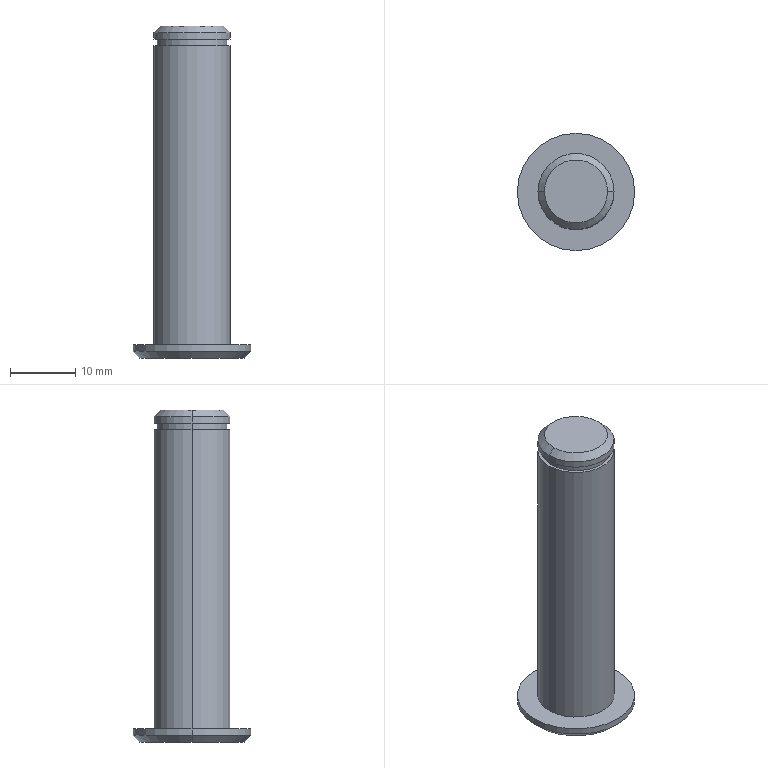Part | SolidWorks | features ICE 3, Chamfer 1, Extrusion 1 | 1 solid | 17 faces | box 18 x 18 x 51 mm | volume 5715 mm3 | cylinder 8 | plane 5 | cone 4 | commonest cylinder face diameters 11.7 x4 10.7 x2 18 x2
STEP:
#1=CARTESIAN_POINT('',(4.85,0.,51.));
#2=VERTEX_POINT('',#1);
#3=CARTESIAN_POINT('',(-4.85,0.,51.));
#4=VERTEX_POINT('',#3);
#5=CARTESIAN_POINT('',(0.,0.,51.));
#6=DIRECTION('',(0.,0.,1.));
#7=DIRECTION('',(1.,0.,0.));
#8=AXIS2_PLACEMENT_3D('',#5,#6,#7);
#9=CIRCLE('',#8,4.85);
#10=EDGE_CURVE('',#2,#4,#9,.T.);
#11=ORIENTED_EDGE('',*,*,#10,.F.);
#12=CARTESIAN_POINT('',(5.85,0.,50.));
#13=VERTEX_POINT('',#12);
#14=CARTESIAN_POINT('',(4.85,0.,51.));
#15=DIRECTION('',(0.7071,0.,-0.7071));
#16=VECTOR('',#15,1000.);
#17=LINE('',#14,#16);
#18=EDGE_CURVE('',#2,#13,#17,.T.);
#19=ORIENTED_EDGE('',*,*,#18,.T.);
#20=CARTESIAN_POINT('',(-5.85,0.,50.));
#21=VERTEX_POINT('',#20);
#22=CARTESIAN_POINT('',(0.,0.,50.));
#23=DIRECTION('',(0.,0.,-1.));
#24=DIRECTION('',(1.,0.,0.));
#25=AXIS2_PLACEMENT_3D('',#22,#23,#24);
#26=CIRCLE('',#25,5.85);
#27=EDGE_CURVE('',#21,#13,#26,.T.);
#28=ORIENTED_EDGE('',*,*,#27,.F.);
#29=CARTESIAN_POINT('',(-4.85,0.,51.));
#30=DIRECTION('',(-0.7071,0.,-0.7071));
#31=VECTOR('',#30,1000.);
#32=LINE('',#29,#31);
#33=EDGE_CURVE('',#4,#21,#32,.T.);
#34=ORIENTED_EDGE('',*,*,#33,.F.);
#35=EDGE_LOOP('',(#11,#19,#28,#34));
#36=FACE_OUTER_BOUND('',#35,.T.);
#37=CARTESIAN_POINT('',(0.,0.,51.));
#38=DIRECTION('',(0.,0.,-1.));
#39=DIRECTION('',(-1.,0.,0.));
#40=AXIS2_PLACEMENT_3D('',#37,#38,#39);
#41=CONICAL_SURFACE('',#40,4.85,0.7854);
#42=ADVANCED_FACE('',(#36),#41,.T.);
#43=CARTESIAN_POINT('',(-8.,0.,0.));
#44=VERTEX_POINT('',#43);
#45=CARTESIAN_POINT('',(8.,0.,0.));
#46=VERTEX_POINT('',#45);
#47=CARTESIAN_POINT('',(0.,0.,0.));
#48=DIRECTION('',(0.,0.,-1.));
#49=DIRECTION('',(1.,0.,0.));
#50=AXIS2_PLACEMENT_3D('',#47,#48,#49);
#51=CIRCLE('',#50,8.);
#52=EDGE_CURVE('',#44,#46,#51,.T.);
#53=ORIENTED_EDGE('',*,*,#52,.F.);
#54=CARTESIAN_POINT('',(-9.,0.,1.));
#55=VERTEX_POINT('',#54);
#56=CARTESIAN_POINT('',(-9.,0.,1.));
#57=DIRECTION('',(-0.7071,0.,0.7071));
#58=VECTOR('',#57,1000.);
#59=LINE('',#56,#58);
#60=EDGE_CURVE('',#44,#55,#59,.T.);
#61=ORIENTED_EDGE('',*,*,#60,.T.);
#62=CARTESIAN_POINT('',(9.,0.,1.));
#63=VERTEX_POINT('',#62);
#64=CARTESIAN_POINT('',(0.,0.,1.));
#65=DIRECTION('',(0.,0.,1.));
#66=DIRECTION('',(1.,0.,0.));
#67=AXIS2_PLACEMENT_3D('',#64,#65,#66);
#68=CIRCLE('',#67,9.);
#69=EDGE_CURVE('',#63,#55,#68,.T.);
#70=ORIENTED_EDGE('',*,*,#69,.F.);
#71=CARTESIAN_POINT('',(9.,0.,1.));
#72=DIRECTION('',(0.7071,0.,0.7071));
#73=VECTOR('',#72,1000.);
#74=LINE('',#71,#73);
#75=EDGE_CURVE('',#46,#63,#74,.T.);
#76=ORIENTED_EDGE('',*,*,#75,.F.);
#77=EDGE_LOOP('',(#53,#61,#70,#76));
#78=FACE_OUTER_BOUND('',#77,.T.);
#79=CARTESIAN_POINT('',(0.,0.,1.));
#80=DIRECTION('',(0.,0.,1.));
#81=DIRECTION('',(1.,0.,0.));
#82=AXIS2_PLACEMENT_3D('',#79,#80,#81);
#83=CONICAL_SURFACE('',#82,9.,0.7854);
#84=ADVANCED_FACE('',(#78),#83,.T.);
#85=ORIENTED_EDGE('',*,*,#27,.T.);
#86=CARTESIAN_POINT('',(5.85,0.,49.));
#87=VERTEX_POINT('',#86);
#88=CARTESIAN_POINT('',(5.85,0.,51.));
#89=DIRECTION('',(0.,0.,-1.));
#90=VECTOR('',#89,1000.);
#91=LINE('',#88,#90);
#92=EDGE_CURVE('',#13,#87,#91,.T.);
#93=ORIENTED_EDGE('',*,*,#92,.T.);
#94=CARTESIAN_POINT('',(-5.85,0.,49.));
#95=VERTEX_POINT('',#94);
#96=CARTESIAN_POINT('',(0.,0.,49.));
#97=DIRECTION('',(0.,0.,1.));
#98=DIRECTION('',(1.,0.,0.));
#99=AXIS2_PLACEMENT_3D('',#96,#97,#98);
#100=CIRCLE('',#99,5.85);
#101=EDGE_CURVE('',#87,#95,#100,.T.);
#102=ORIENTED_EDGE('',*,*,#101,.T.);
#103=CARTESIAN_POINT('',(-5.85,0.,51.));
#104=DIRECTION('',(0.,0.,-1.));
#105=VECTOR('',#104,1000.);
#106=LINE('',#103,#105);
#107=EDGE_CURVE('',#21,#95,#106,.T.);
#108=ORIENTED_EDGE('',*,*,#107,.F.);
#109=EDGE_LOOP('',(#85,#93,#102,#108));
#110=FACE_OUTER_BOUND('',#109,.T.);
#111=CARTESIAN_POINT('',(0.,0.,51.));
#112=DIRECTION('',(0.,0.,-1.));
#113=DIRECTION('',(-1.,0.,0.));
#114=AXIS2_PLACEMENT_3D('',#111,#112,#113);
#115=CYLINDRICAL_SURFACE('',#114,5.85);
#116=ADVANCED_FACE('',(#110),#115,.T.);
#117=CARTESIAN_POINT('',(5.35,0.,49.));
#118=VERTEX_POINT('',#117);
#119=CARTESIAN_POINT('',(-5.35,0.,49.));
#120=VERTEX_POINT('',#119);
#121=CARTESIAN_POINT('',(0.,0.,49.));
#122=DIRECTION('',(0.,0.,1.));
#123=DIRECTION('',(1.,0.,0.));
#124=AXIS2_PLACEMENT_3D('',#121,#122,#123);
#125=CIRCLE('',#124,5.35);
#126=EDGE_CURVE('',#118,#120,#125,.T.);
#127=ORIENTED_EDGE('',*,*,#126,.F.);
#128=CARTESIAN_POINT('',(5.35,0.,48.));
#129=VERTEX_POINT('',#128);
#130=CARTESIAN_POINT('',(5.35,0.,49.));
#131=DIRECTION('',(0.,0.,-1.));
#132=VECTOR('',#131,1000.);
#133=LINE('',#130,#132);
#134=EDGE_CURVE('',#118,#129,#133,.T.);
#135=ORIENTED_EDGE('',*,*,#134,.T.);
#136=CARTESIAN_POINT('',(-5.35,0.,48.));
#137=VERTEX_POINT('',#136);
#138=CARTESIAN_POINT('',(0.,0.,48.));
#139=DIRECTION('',(0.,0.,1.));
#140=DIRECTION('',(1.,0.,0.));
#141=AXIS2_PLACEMENT_3D('',#138,#139,#140);
#142=CIRCLE('',#141,5.35);
#143=EDGE_CURVE('',#129,#137,#142,.T.);
#144=ORIENTED_EDGE('',*,*,#143,.T.);
#145=CARTESIAN_POINT('',(-5.35,0.,49.));
#146=DIRECTION('',(0.,0.,-1.));
#147=VECTOR('',#146,1000.);
#148=LINE('',#145,#147);
#149=EDGE_CURVE('',#120,#137,#148,.T.);
#150=ORIENTED_EDGE('',*,*,#149,.F.);
#151=EDGE_LOOP('',(#127,#135,#144,#150));
#152=FACE_OUTER_BOUND('',#151,.T.);
#153=CARTESIAN_POINT('',(0.,0.,49.));
#154=DIRECTION('',(0.,0.,-1.));
#155=DIRECTION('',(-1.,0.,0.));
#156=AXIS2_PLACEMENT_3D('',#153,#154,#155);
#157=CYLINDRICAL_SURFACE('',#156,5.35);
#158=ADVANCED_FACE('',(#152),#157,.T.);
#159=CARTESIAN_POINT('',(5.85,0.,48.));
#160=VERTEX_POINT('',#159);
#161=CARTESIAN_POINT('',(-5.85,0.,48.));
#162=VERTEX_POINT('',#161);
#163=CARTESIAN_POINT('',(0.,0.,48.));
#164=DIRECTION('',(0.,0.,1.));
#165=DIRECTION('',(1.,0.,0.));
#166=AXIS2_PLACEMENT_3D('',#163,#164,#165);
#167=CIRCLE('',#166,5.85);
#168=EDGE_CURVE('',#160,#162,#167,.T.);
#169=ORIENTED_EDGE('',*,*,#168,.F.);
#170=CARTESIAN_POINT('',(5.85,0.,2.));
#171=VERTEX_POINT('',#170);
#172=CARTESIAN_POINT('',(5.85,0.,48.));
#173=DIRECTION('',(0.,0.,-1.));
#174=VECTOR('',#173,1000.);
#175=LINE('',#172,#174);
#176=EDGE_CURVE('',#160,#171,#175,.T.);
#177=ORIENTED_EDGE('',*,*,#176,.T.);
#178=CARTESIAN_POINT('',(-5.85,0.,2.));
#179=VERTEX_POINT('',#178);
#180=CARTESIAN_POINT('',(0.,0.,2.));
#181=DIRECTION('',(0.,0.,1.));
#182=DIRECTION('',(1.,0.,0.));
#183=AXIS2_PLACEMENT_3D('',#180,#181,#182);
#184=CIRCLE('',#183,5.85);
#185=EDGE_CURVE('',#171,#179,#184,.T.);
#186=ORIENTED_EDGE('',*,*,#185,.T.);
#187=CARTESIAN_POINT('',(-5.85,0.,48.));
#188=DIRECTION('',(0.,0.,-1.));
#189=VECTOR('',#188,1000.);
#190=LINE('',#187,#189);
#191=EDGE_CURVE('',#162,#179,#190,.T.);
#192=ORIENTED_EDGE('',*,*,#191,.F.);
#193=EDGE_LOOP('',(#169,#177,#186,#192));
#194=FACE_OUTER_BOUND('',#193,.T.);
#195=CARTESIAN_POINT('',(0.,0.,48.));
#196=DIRECTION('',(0.,0.,-1.));
#197=DIRECTION('',(-1.,0.,0.));
#198=AXIS2_PLACEMENT_3D('',#195,#196,#197);
#199=CYLINDRICAL_SURFACE('',#198,5.85);
#200=ADVANCED_FACE('',(#194),#199,.T.);
#201=CARTESIAN_POINT('',(9.,0.,2.));
#202=VERTEX_POINT('',#201);
#203=CARTESIAN_POINT('',(-9.,0.,2.));
#204=VERTEX_POINT('',#203);
#205=CARTESIAN_POINT('',(0.,0.,2.));
#206=DIRECTION('',(0.,0.,1.));
#207=DIRECTION('',(1.,0.,0.));
#208=AXIS2_PLACEMENT_3D('',#205,#206,#207);
#209=CIRCLE('',#208,9.);
#210=EDGE_CURVE('',#202,#204,#209,.T.);
#211=ORIENTED_EDGE('',*,*,#210,.F.);
#212=CARTESIAN_POINT('',(9.,0.,2.));
#213=DIRECTION('',(0.,0.,-1.));
#214=VECTOR('',#213,1000.);
#215=LINE('',#212,#214);
#216=EDGE_CURVE('',#202,#63,#215,.T.);
#217=ORIENTED_EDGE('',*,*,#216,.T.);
#218=ORIENTED_EDGE('',*,*,#69,.T.);
#219=CARTESIAN_POINT('',(-9.,0.,2.));
#220=DIRECTION('',(0.,0.,-1.));
#221=VECTOR('',#220,1000.);
#222=LINE('',#219,#221);
#223=EDGE_CURVE('',#204,#55,#222,.T.);
#224=ORIENTED_EDGE('',*,*,#223,.F.);
#225=EDGE_LOOP('',(#211,#217,#218,#224));
#226=FACE_OUTER_BOUND('',#225,.T.);
#227=CARTESIAN_POINT('',(0.,0.,2.));
#228=DIRECTION('',(0.,0.,-1.));
#229=DIRECTION('',(-1.,0.,0.));
#230=AXIS2_PLACEMENT_3D('',#227,#228,#229);
#231=CYLINDRICAL_SURFACE('',#230,9.);
#232=ADVANCED_FACE('',(#226),#231,.T.);
#233=ORIENTED_EDGE('',*,*,#216,.F.);
#234=CARTESIAN_POINT('',(0.,0.,2.));
#235=DIRECTION('',(0.,0.,1.));
#236=DIRECTION('',(1.,0.,0.));
#237=AXIS2_PLACEMENT_3D('',#234,#235,#236);
#238=CIRCLE('',#237,9.);
#239=EDGE_CURVE('',#204,#202,#238,.T.);
#240=ORIENTED_EDGE('',*,*,#239,.F.);
#241=ORIENTED_EDGE('',*,*,#223,.T.);
#242=CARTESIAN_POINT('',(0.,0.,1.));
#243=DIRECTION('',(0.,0.,1.));
#244=DIRECTION('',(1.,0.,0.));
#245=AXIS2_PLACEMENT_3D('',#242,#243,#244);
#246=CIRCLE('',#245,9.);
#247=EDGE_CURVE('',#55,#63,#246,.T.);
#248=ORIENTED_EDGE('',*,*,#247,.T.);
#249=EDGE_LOOP('',(#233,#240,#241,#248));
#250=FACE_OUTER_BOUND('',#249,.T.);
#251=CARTESIAN_POINT('',(0.,0.,2.));
#252=DIRECTION('',(0.,0.,-1.));
#253=DIRECTION('',(-1.,0.,0.));
#254=AXIS2_PLACEMENT_3D('',#251,#252,#253);
#255=CYLINDRICAL_SURFACE('',#254,9.);
#256=ADVANCED_FACE('',(#250),#255,.T.);
#257=CARTESIAN_POINT('',(0.,0.,2.));
#258=DIRECTION('',(0.,0.,1.));
#259=DIRECTION('',(1.,0.,0.));
#260=AXIS2_PLACEMENT_3D('',#257,#258,#259);
#261=CIRCLE('',#260,5.85);
#262=EDGE_CURVE('',#179,#171,#261,.T.);
#263=ORIENTED_EDGE('',*,*,#262,.F.);
#264=ORIENTED_EDGE('',*,*,#185,.F.);
#265=EDGE_LOOP('',(#263,#264));
#266=FACE_BOUND('',#265,.T.);
#267=ORIENTED_EDGE('',*,*,#239,.T.);
#268=ORIENTED_EDGE('',*,*,#210,.T.);
#269=EDGE_LOOP('',(#267,#268));
#270=FACE_OUTER_BOUND('',#269,.T.);
#271=CARTESIAN_POINT('',(0.,0.,2.));
#272=DIRECTION('',(0.,0.,1.));
#273=DIRECTION('',(1.,0.,0.));
#274=AXIS2_PLACEMENT_3D('',#271,#272,#273);
#275=PLANE('',#274);
#276=ADVANCED_FACE('',(#266,#270),#275,.T.);
#277=CARTESIAN_POINT('',(0.,0.,0.));
#278=DIRECTION('',(0.,0.,-1.));
#279=DIRECTION('',(1.,0.,0.));
#280=AXIS2_PLACEMENT_3D('',#277,#278,#279);
#281=CIRCLE('',#280,8.);
#282=EDGE_CURVE('',#46,#44,#281,.T.);
#283=ORIENTED_EDGE('',*,*,#282,.T.);
#284=ORIENTED_EDGE('',*,*,#52,.T.);
#285=EDGE_LOOP('',(#283,#284));
#286=FACE_OUTER_BOUND('',#285,.T.);
#287=CARTESIAN_POINT('',(0.,0.,0.));
#288=DIRECTION('',(0.,0.,1.));
#289=DIRECTION('',(1.,0.,0.));
#290=AXIS2_PLACEMENT_3D('',#287,#288,#289);
#291=PLANE('',#290);
#292=ADVANCED_FACE('',(#286),#291,.F.);
#293=ORIENTED_EDGE('',*,*,#176,.F.);
#294=CARTESIAN_POINT('',(0.,0.,48.));
#295=DIRECTION('',(0.,0.,1.));
#296=DIRECTION('',(1.,0.,0.));
#297=AXIS2_PLACEMENT_3D('',#294,#295,#296);
#298=CIRCLE('',#297,5.85);
#299=EDGE_CURVE('',#162,#160,#298,.T.);
#300=ORIENTED_EDGE('',*,*,#299,.F.);
#301=ORIENTED_EDGE('',*,*,#191,.T.);
#302=ORIENTED_EDGE('',*,*,#262,.T.);
#303=EDGE_LOOP('',(#293,#300,#301,#302));
#304=FACE_OUTER_BOUND('',#303,.T.);
#305=CARTESIAN_POINT('',(0.,0.,48.));
#306=DIRECTION('',(0.,0.,-1.));
#307=DIRECTION('',(-1.,0.,0.));
#308=AXIS2_PLACEMENT_3D('',#305,#306,#307);
#309=CYLINDRICAL_SURFACE('',#308,5.85);
#310=ADVANCED_FACE('',(#304),#309,.T.);
#311=CARTESIAN_POINT('',(0.,0.,48.));
#312=DIRECTION('',(0.,0.,1.));
#313=DIRECTION('',(1.,0.,0.));
#314=AXIS2_PLACEMENT_3D('',#311,#312,#313);
#315=CIRCLE('',#314,5.35);
#316=EDGE_CURVE('',#137,#129,#315,.T.);
#317=ORIENTED_EDGE('',*,*,#316,.F.);
#318=ORIENTED_EDGE('',*,*,#143,.F.);
#319=EDGE_LOOP('',(#317,#318));
#320=FACE_BOUND('',#319,.T.);
#321=ORIENTED_EDGE('',*,*,#299,.T.);
#322=ORIENTED_EDGE('',*,*,#168,.T.);
#323=EDGE_LOOP('',(#321,#322));
#324=FACE_OUTER_BOUND('',#323,.T.);
#325=CARTESIAN_POINT('',(0.,0.,48.));
#326=DIRECTION('',(0.,0.,1.));
#327=DIRECTION('',(1.,0.,0.));
#328=AXIS2_PLACEMENT_3D('',#325,#326,#327);
#329=PLANE('',#328);
#330=ADVANCED_FACE('',(#320,#324),#329,.T.);
#331=ORIENTED_EDGE('',*,*,#134,.F.);
#332=CARTESIAN_POINT('',(0.,0.,49.));
#333=DIRECTION('',(0.,0.,1.));
#334=DIRECTION('',(1.,0.,0.));
#335=AXIS2_PLACEMENT_3D('',#332,#333,#334);
#336=CIRCLE('',#335,5.35);
#337=EDGE_CURVE('',#120,#118,#336,.T.);
#338=ORIENTED_EDGE('',*,*,#337,.F.);
#339=ORIENTED_EDGE('',*,*,#149,.T.);
#340=ORIENTED_EDGE('',*,*,#316,.T.);
#341=EDGE_LOOP('',(#331,#338,#339,#340));
#342=FACE_OUTER_BOUND('',#341,.T.);
#343=CARTESIAN_POINT('',(0.,0.,49.));
#344=DIRECTION('',(0.,0.,-1.));
#345=DIRECTION('',(-1.,0.,0.));
#346=AXIS2_PLACEMENT_3D('',#343,#344,#345);
#347=CYLINDRICAL_SURFACE('',#346,5.35);
#348=ADVANCED_FACE('',(#342),#347,.T.);
#349=ORIENTED_EDGE('',*,*,#92,.F.);
#350=CARTESIAN_POINT('',(0.,0.,50.));
#351=DIRECTION('',(0.,0.,-1.));
#352=DIRECTION('',(1.,0.,0.));
#353=AXIS2_PLACEMENT_3D('',#350,#351,#352);
#354=CIRCLE('',#353,5.85);
#355=EDGE_CURVE('',#13,#21,#354,.T.);
#356=ORIENTED_EDGE('',*,*,#355,.T.);
#357=ORIENTED_EDGE('',*,*,#107,.T.);
#358=CARTESIAN_POINT('',(0.,0.,49.));
#359=DIRECTION('',(0.,0.,1.));
#360=DIRECTION('',(1.,0.,0.));
#361=AXIS2_PLACEMENT_3D('',#358,#359,#360);
#362=CIRCLE('',#361,5.85);
#363=EDGE_CURVE('',#95,#87,#362,.T.);
#364=ORIENTED_EDGE('',*,*,#363,.T.);
#365=EDGE_LOOP('',(#349,#356,#357,#364));
#366=FACE_OUTER_BOUND('',#365,.T.);
#367=CARTESIAN_POINT('',(0.,0.,51.));
#368=DIRECTION('',(0.,0.,-1.));
#369=DIRECTION('',(-1.,0.,0.));
#370=AXIS2_PLACEMENT_3D('',#367,#368,#369);
#371=CYLINDRICAL_SURFACE('',#370,5.85);
#372=ADVANCED_FACE('',(#366),#371,.T.);
#373=CARTESIAN_POINT('',(0.,0.,51.));
#374=DIRECTION('',(0.,0.,1.));
#375=DIRECTION('',(1.,0.,0.));
#376=AXIS2_PLACEMENT_3D('',#373,#374,#375);
#377=CIRCLE('',#376,4.85);
#378=EDGE_CURVE('',#4,#2,#377,.T.);
#379=ORIENTED_EDGE('',*,*,#378,.T.);
#380=ORIENTED_EDGE('',*,*,#10,.T.);
#381=EDGE_LOOP('',(#379,#380));
#382=FACE_OUTER_BOUND('',#381,.T.);
#383=CARTESIAN_POINT('',(0.,0.,51.));
#384=DIRECTION('',(0.,0.,1.));
#385=DIRECTION('',(1.,0.,0.));
#386=AXIS2_PLACEMENT_3D('',#383,#384,#385);
#387=PLANE('',#386);
#388=ADVANCED_FACE('',(#382),#387,.T.);
#389=ORIENTED_EDGE('',*,*,#337,.T.);
#390=ORIENTED_EDGE('',*,*,#126,.T.);
#391=EDGE_LOOP('',(#389,#390));
#392=FACE_BOUND('',#391,.T.);
#393=ORIENTED_EDGE('',*,*,#363,.F.);
#394=ORIENTED_EDGE('',*,*,#101,.F.);
#395=EDGE_LOOP('',(#393,#394));
#396=FACE_OUTER_BOUND('',#395,.T.);
#397=CARTESIAN_POINT('',(0.,0.,49.));
#398=DIRECTION('',(0.,0.,1.));
#399=DIRECTION('',(1.,0.,0.));
#400=AXIS2_PLACEMENT_3D('',#397,#398,#399);
#401=PLANE('',#400);
#402=ADVANCED_FACE('',(#392,#396),#401,.F.);
#403=ORIENTED_EDGE('',*,*,#60,.F.);
#404=ORIENTED_EDGE('',*,*,#282,.F.);
#405=ORIENTED_EDGE('',*,*,#75,.T.);
#406=ORIENTED_EDGE('',*,*,#247,.F.);
#407=EDGE_LOOP('',(#403,#404,#405,#406));
#408=FACE_OUTER_BOUND('',#407,.T.);
#409=CARTESIAN_POINT('',(0.,0.,1.));
#410=DIRECTION('',(0.,0.,1.));
#411=DIRECTION('',(1.,0.,0.));
#412=AXIS2_PLACEMENT_3D('',#409,#410,#411);
#413=CONICAL_SURFACE('',#412,9.,0.7854);
#414=ADVANCED_FACE('',(#408),#413,.T.);
#415=ORIENTED_EDGE('',*,*,#18,.F.);
#416=ORIENTED_EDGE('',*,*,#378,.F.);
#417=ORIENTED_EDGE('',*,*,#33,.T.);
#418=ORIENTED_EDGE('',*,*,#355,.F.);
#419=EDGE_LOOP('',(#415,#416,#417,#418));
#420=FACE_OUTER_BOUND('',#419,.T.);
#421=CARTESIAN_POINT('',(0.,0.,51.));
#422=DIRECTION('',(0.,0.,-1.));
#423=DIRECTION('',(-1.,0.,0.));
#424=AXIS2_PLACEMENT_3D('',#421,#422,#423);
#425=CONICAL_SURFACE('',#424,4.85,0.7854);
#426=ADVANCED_FACE('',(#420),#425,.T.);
#427=CLOSED_SHELL('',(#42,#84,#116,#158,#200,#232,#256,#276,#292,#310,#330,#348,#372,#388,#402,#414,#426));
#428=MANIFOLD_SOLID_BREP('',#427);
#429=CARTESIAN_POINT('',(0.,0.,0.));
#430=DIRECTION('',(0.,0.,1.));
#431=DIRECTION('',(1.,0.,0.));
#432=AXIS2_PLACEMENT_3D('',#429,#430,#431);
#433=(LENGTH_UNIT()NAMED_UNIT(*)SI_UNIT(.MILLI.,.METRE.));
#434=UNCERTAINTY_MEASURE_WITH_UNIT(LENGTH_MEASURE(0.00001),#433,'','');
#435=(NAMED_UNIT(*)PLANE_ANGLE_UNIT()SI_UNIT($,.RADIAN.));
#436=(NAMED_UNIT(*)SI_UNIT($,.STERADIAN.)SOLID_ANGLE_UNIT());
#437=(GEOMETRIC_REPRESENTATION_CONTEXT(3)GLOBAL_UNCERTAINTY_ASSIGNED_CONTEXT((#434))GLOBAL_UNIT_ASSIGNED_CONTEXT((#433,#435,#436))REPRESENTATION_CONTEXT('',''));
#438=ADVANCED_BREP_SHAPE_REPRESENTATION('',(#428,#432),#437);